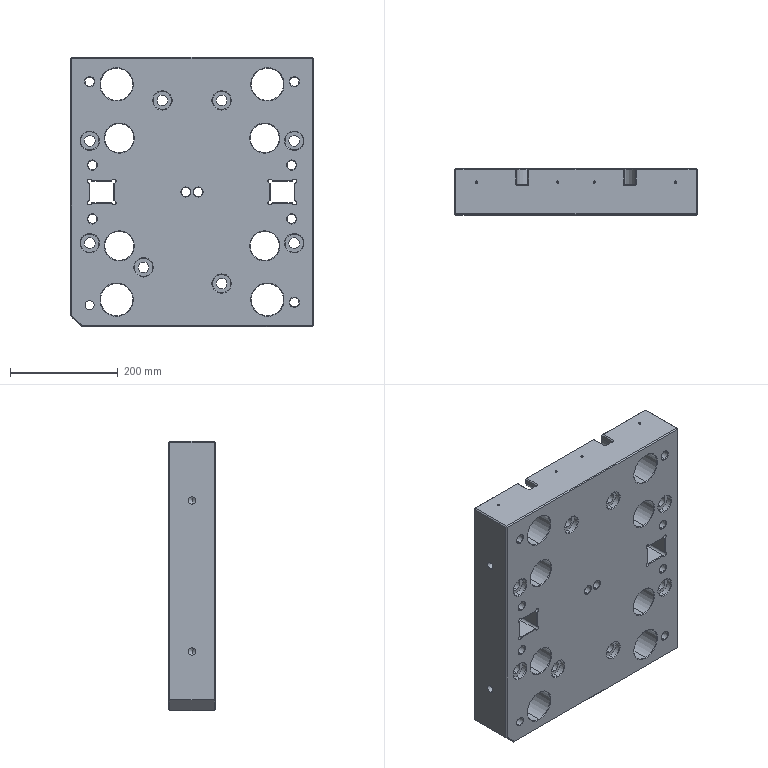Part | STEP file | Manifold - torre - 1 cav | 1 solid | 775 faces | box 450 x 86 x 500 mm | volume 13913038 mm3 | cylinder 284 | cone 212 | plane 208 | torus 57 | spline 14 | commonest cylinder face diameters 20 x37 10.2 x26 4.2 x22 17 x20 60 x20 1 x18